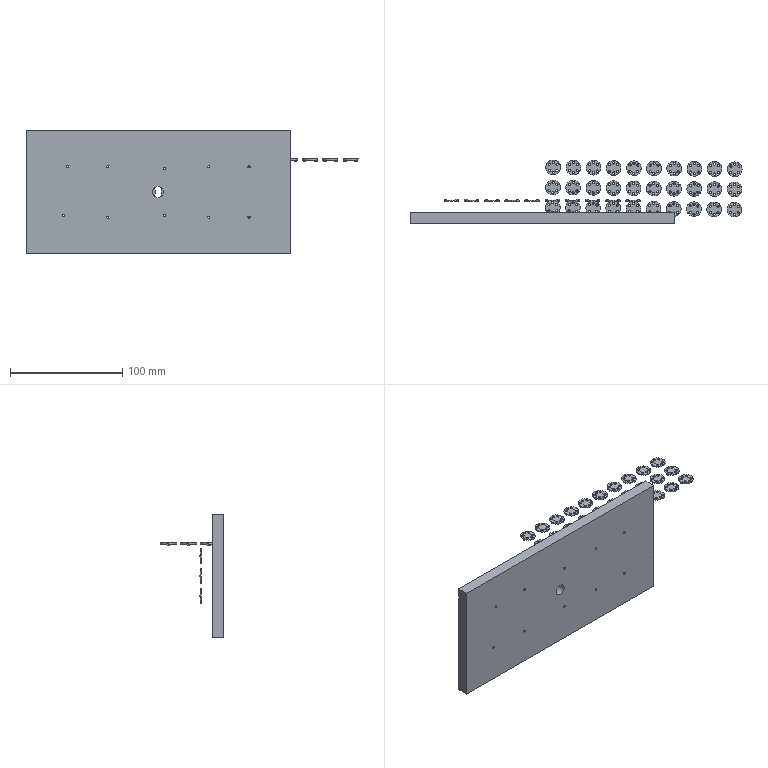NC program | NX | posted with a generic post | part box 296.27 x 56.878 x 110 mm
Lines 2497 to 3687 of 20851:
(DRILLING , TOOL : DK-Ø3)
N4992 T04 M6
N4994 G53
N4996 G17 G0 G90 X6.362 Y20.807 B0. C0. S1500 M3
N4998 G43 Z5. H4
N5000 G94 G81 G99 Z-1. F100. R1.
N5002 G0 Z5.
N5004 G81 X6.321 Y15.012 Z-1. R1.
N5006 G0 Z5.
N5008 G81 X9.826 Y22.378 Z-1. R1.
N5010 G0 Z5.
N5012 G81 X9.731 Y13.378 Z-1. R1.
N5014 G0 Z5.
N5016 G81 X13.195 Y14.949 Z-1. R1.
N5018 G0 Z5.
N5020 G81 X13.276 Y20.724 Z-1. R1.
N5022 G0 Z5.
N5024 G81 X24.361 Y20.617 Z-1. R1.
N5026 G0 Z5.
N5028 G81 X24.32 Y14.822 Z-1. R1.
N5030 G0 Z5.
N5032 G81 X27.825 Y22.188 Z-1. R1.
N5034 G0 Z5.
N5036 G81 X27.73 Y13.189 Z-1. R1.
N5038 G0 Z5.
N5040 G81 X31.194 Y14.76 Z-1. R1.
N5042 G0 Z5.
N5044 G81 X31.275 Y20.534 Z-1. R1.
N5046 G0 Z5.
N5048 G81 X42.36 Y20.427 Z-1. R1.
N5050 G0 Z5.
N5052 G81 X42.319 Y14.633 Z-1. R1.
N5054 G0 Z5.
N5056 G81 X45.824 Y21.998 Z-1. R1.
N5058 G0 Z5.
N5060 G81 X45.729 Y12.999 Z-1. R1.
N5062 G0 Z5.
N5064 G81 X49.193 Y14.57 Z-1. R1.
N5066 G0 Z5.
N5068 G81 X49.274 Y20.345 Z-1. R1.
N5070 G0 Z5.
N5072 G81 X60.359 Y20.238 Z-1. R1.
N5074 G0 Z5.
N5076 G81 X60.318 Y14.443 Z-1. R1.
N5078 G0 Z5.
N5080 G81 X63.823 Y21.809 Z-1. R1.
N5082 G0 Z5.
N5084 G81 X63.728 Y12.809 Z-1. R1.
N5086 G0 Z5.
N5088 G81 X67.192 Y14.38 Z-1. R1.
N5090 G0 Z5.
N5092 G81 X67.273 Y20.155 Z-1. R1.
N5094 G0 Z5.
N5096 G81 X78.358 Y20.048 Z-1. R1.
N5098 G0 Z5.
N5100 G81 X78.317 Y14.253 Z-1. R1.
N5102 G0 Z5.
N5104 G81 X81.822 Y21.619 Z-1. R1.
N5106 G0 Z5.
N5108 G81 X81.727 Y12.62 Z-1. R1.
N5110 G0 Z5.
N5112 G81 X85.191 Y14.191 Z-1. R1.
N5114 G0 Z5.
N5116 G81 X85.272 Y19.966 Z-1. R1.
N5118 G0 Z5.
N5120 G81 X96.357 Y19.859 Z-1. R1.
N5122 G0 Z5.
N5124 G81 X96.316 Y14.064 Z-1. R1.
N5126 G0 Z5.
N5128 G81 X99.821 Y21.43 Z-1. R1.
N5130 G0 Z5.
N5132 G81 X99.726 Y12.43 Z-1. R1.
N5134 G0 Z5.
N5136 G81 X103.19 Y14.001 Z-1. R1.
N5138 G0 Z5.
N5140 G81 X103.271 Y19.776 Z-1. R1.
N5142 G0 Z5.
N5144 G81 X114.356 Y19.669 Z-1. R1.
N5146 G0 Z5.
N5148 G81 X114.315 Y13.874 Z-1. R1.
N5150 G0 Z5.
N5152 G81 X117.82 Y21.24 Z-1. R1.
N5154 G0 Z5.
N5156 G81 X117.725 Y12.24 Z-1. R1.
N5158 G0 Z5.
N5160 G81 X121.189 Y13.811 Z-1. R1.
N5162 G0 Z5.
N5164 G81 X121.27 Y19.586 Z-1. R1.
N5166 G0 Z5.
N5168 G81 X132.355 Y19.479 Z-1. R1.
N5170 G0 Z5.
N5172 G81 X132.314 Y13.685 Z-1. R1.
N5174 G0 Z5.
N5176 G81 X135.819 Y21.05 Z-1. R1.
N5178 G0 Z5.
N5180 G81 X135.724 Y12.051 Z-1. R1.
N5182 G0 Z5.
N5184 G81 X139.188 Y13.622 Z-1. R1.
N5186 G0 Z5.
N5188 G81 X139.269 Y19.397 Z-1. R1.
N5190 G0 Z5.
N5192 G81 X150.354 Y19.29 Z-1. R1.
N5194 G0 Z5.
N5196 G81 X150.313 Y13.495 Z-1. R1.
N5198 G0 Z5.
N5200 G81 X153.818 Y20.861 Z-1. R1.
N5202 G0 Z5.
N5204 G81 X153.723 Y11.861 Z-1. R1.
N5206 G0 Z5.
N5208 G81 X157.187 Y13.432 Z-1. R1.
N5210 G0 Z5.
N5212 G81 X157.268 Y19.207 Z-1. R1.
N5214 G0 Z5.
N5216 G81 X168.353 Y19.1 Z-1. R1.
N5218 G0 Z5.
N5220 G81 X168.312 Y13.305 Z-1. R1.
N5222 G0 Z5.
N5224 G81 X171.817 Y20.671 Z-1. R1.
N5226 G0 Z5.
N5228 G81 X171.722 Y11.672 Z-1. R1.
N5230 G0 Z5.
N5232 G81 X175.186 Y13.243 Z-1. R1.
N5234 G0 Z5.
N5236 G81 X175.267 Y19.017 Z-1. R1.
N5238 G0 Z5.
N5240 G81 X168.163 Y1.101 Z-1. R1.
N5242 G0 Z5.
N5244 G81 X168.122 Y-4.694 Z-1. R1.
N5246 G0 Z5.
N5248 G81 X171.627 Y2.672 Z-1. R1.
N5250 G0 Z5.
N5252 G81 X171.533 Y-6.327 Z-1. R1.
N5254 G0 Z5.
N5256 G81 X174.996 Y-4.756 Z-1. R1.
N5258 G0 Z5.
N5260 G81 X175.077 Y1.018 Z-1. R1.
N5262 G0 Z5.
N5264 G81 X150.164 Y1.291 Z-1. R1.
N5266 G0 Z5.
N5268 G81 X150.123 Y-4.504 Z-1. R1.
N5270 G0 Z5.
N5272 G81 X153.628 Y2.862 Z-1. R1.
N5274 G0 Z5.
N5276 G81 X153.534 Y-6.138 Z-1. R1.
N5278 G0 Z5.
N5280 G81 X156.997 Y-4.567 Z-1. R1.
N5282 G0 Z5.
N5284 G81 X157.078 Y1.208 Z-1. R1.
N5286 G0 Z5.
N5288 G81 X132.165 Y1.48 Z-1. R1.
N5290 G0 Z5.
N5292 G81 X132.124 Y-4.314 Z-1. R1.
N5294 G0 Z5.
N5296 G81 X135.629 Y3.051 Z-1. R1.
N5298 G0 Z5.
N5300 G81 X135.535 Y-5.948 Z-1. R1.
N5302 G0 Z5.
N5304 G81 X138.998 Y-4.377 Z-1. R1.
N5306 G0 Z5.
N5308 G81 X139.079 Y1.398 Z-1. R1.
N5310 G0 Z5.
N5312 G81 X114.166 Y1.67 Z-1. R1.
N5314 G0 Z5.
N5316 G81 X114.125 Y-4.125 Z-1. R1.
N5318 G0 Z5.
N5320 G81 X117.63 Y3.241 Z-1. R1.
N5322 G0 Z5.
N5324 G81 X117.536 Y-5.759 Z-1. R1.
N5326 G0 Z5.
N5328 G81 X120.999 Y-4.188 Z-1. R1.
N5330 G0 Z5.
N5332 G81 X121.08 Y1.587 Z-1. R1.
N5334 G0 Z5.
N5336 G81 X96.167 Y1.86 Z-1. R1.
N5338 G0 Z5.
N5340 G81 X96.126 Y-3.935 Z-1. R1.
N5342 G0 Z5.
N5344 G81 X99.631 Y3.431 Z-1. R1.
N5346 G0 Z5.
N5348 G81 X99.537 Y-5.569 Z-1. R1.
N5350 G0 Z5.
N5352 G81 X103. Y-3.998 Z-1. R1.
N5354 G0 Z5.
N5356 G81 X103.081 Y1.777 Z-1. R1.
N5358 G0 Z5.
N5360 G81 X78.168 Y2.049 Z-1. R1.
N5362 G0 Z5.
N5364 G81 X78.127 Y-3.746 Z-1. R1.
N5366 G0 Z5.
N5368 G81 X81.632 Y3.62 Z-1. R1.
N5370 G0 Z5.
N5372 G81 X81.538 Y-5.379 Z-1. R1.
N5374 G0 Z5.
N5376 G81 X85.001 Y-3.808 Z-1. R1.
N5378 G0 Z5.
N5380 G81 X85.082 Y1.967 Z-1. R1.
N5382 G0 Z5.
N5384 G81 X60.169 Y2.239 Z-1. R1.
N5386 G0 Z5.
N5388 G81 X60.128 Y-3.556 Z-1. R1.
N5390 G0 Z5.
N5392 G81 X63.633 Y3.81 Z-1. R1.
N5394 G0 Z5.
N5396 G81 X63.539 Y-5.19 Z-1. R1.
N5398 G0 Z5.
N5400 G81 X67.002 Y-3.619 Z-1. R1.
N5402 G0 Z5.
N5404 G81 X67.083 Y2.156 Z-1. R1.
N5406 G0 Z5.
N5408 G81 X42.17 Y2.428 Z-1. R1.
N5410 G0 Z5.
N5412 G81 X42.129 Y-3.366 Z-1. R1.
N5414 G0 Z5.
N5416 G81 X45.634 Y3.999 Z-1. R1.
N5418 G0 Z5.
N5420 G81 X45.54 Y-5. Z-1. R1.
N5422 G0 Z5.
N5424 G81 X49.003 Y-3.429 Z-1. R1.
N5426 G0 Z5.
N5428 G81 X49.084 Y2.346 Z-1. R1.
N5430 G0 Z5.
N5432 G81 X24.171 Y2.618 Z-1. R1.
N5434 G0 Z5.
N5436 G81 X24.13 Y-3.177 Z-1. R1.
N5438 G0 Z5.
N5440 G81 X27.635 Y4.189 Z-1. R1.
N5442 G0 Z5.
N5444 G81 X27.541 Y-4.81 Z-1. R1.
N5446 G0 Z5.
N5448 G81 X31.004 Y-3.239 Z-1. R1.
N5450 G0 Z5.
N5452 G81 X31.085 Y2.535 Z-1. R1.
N5454 G0 Z5.
N5456 G81 X6.172 Y2.808 Z-1. R1.
N5458 G0 Z5.
N5460 G81 X6.131 Y-2.987 Z-1. R1.
N5462 G0 Z5.
N5464 G81 X9.636 Y4.379 Z-1. R1.
N5466 G0 Z5.
N5468 G81 X9.542 Y-4.621 Z-1. R1.
N5470 G0 Z5.
N5472 G81 X13.005 Y-3.05 Z-1. R1.
N5474 G0 Z5.
N5476 G81 X13.086 Y2.725 Z-1. R1.
N5478 G0 Z5.
N5480 G81 X5.983 Y-15.191 Z-1. R1.
N5482 G0 Z5.
N5484 G81 X5.942 Y-20.986 Z-1. R1.
N5486 G0 Z5.
N5488 G81 X9.447 Y-13.62 Z-1. R1.
N5490 G0 Z5.
N5492 G81 X9.352 Y-22.62 Z-1. R1.
N5494 G0 Z5.
N5496 G81 X12.816 Y-21.049 Z-1. R1.
N5498 G0 Z5.
N5500 G81 X12.897 Y-15.274 Z-1. R1.
N5502 G0 Z5.
N5504 G81 X23.982 Y-15.381 Z-1. R1.
N5506 G0 Z5.
N5508 G81 X23.941 Y-21.176 Z-1. R1.
N5510 G0 Z5.
N5512 G81 X27.446 Y-13.81 Z-1. R1.
N5514 G0 Z5.
N5516 G81 X27.351 Y-22.809 Z-1. R1.
N5518 G0 Z5.
N5520 G81 X30.815 Y-21.238 Z-1. R1.
N5522 G0 Z5.
N5524 G81 X30.896 Y-15.464 Z-1. R1.
N5526 G0 Z5.
N5528 G81 X41.981 Y-15.571 Z-1. R1.
N5530 G0 Z5.
N5532 G81 X41.94 Y-21.365 Z-1. R1.
N5534 G0 Z5.
N5536 G81 X45.445 Y-14. Z-1. R1.
N5538 G0 Z5.
N5540 G81 X45.35 Y-22.999 Z-1. R1.
N5542 G0 Z5.
N5544 G81 X48.814 Y-21.428 Z-1. R1.
N5546 G0 Z5.
N5548 G81 X48.895 Y-15.653 Z-1. R1.
N5550 G0 Z5.
N5552 G81 X59.98 Y-15.76 Z-1. R1.
N5554 G0 Z5.
N5556 G81 X59.939 Y-21.555 Z-1. R1.
N5558 G0 Z5.
N5560 G81 X63.444 Y-14.189 Z-1. R1.
N5562 G0 Z5.
N5564 G81 X63.349 Y-23.189 Z-1. R1.
N5566 G0 Z5.
N5568 G81 X66.813 Y-21.618 Z-1. R1.
N5570 G0 Z5.
N5572 G81 X66.894 Y-15.843 Z-1. R1.
N5574 G0 Z5.
N5576 G81 X77.979 Y-15.95 Z-1. R1.
N5578 G0 Z5.
N5580 G81 X77.938 Y-21.745 Z-1. R1.
N5582 G0 Z5.
N5584 G81 X81.443 Y-14.379 Z-1. R1.
N5586 G0 Z5.
N5588 G81 X81.348 Y-23.378 Z-1. R1.
N5590 G0 Z5.
N5592 G81 X84.812 Y-21.807 Z-1. R1.
N5594 G0 Z5.
N5596 G81 X84.893 Y-16.032 Z-1. R1.
N5598 G0 Z5.
N5600 G81 X95.978 Y-16.139 Z-1. R1.
N5602 G0 Z5.
N5604 G81 X95.937 Y-21.934 Z-1. R1.
N5606 G0 Z5.
N5608 G81 X99.442 Y-14.568 Z-1. R1.
N5610 G0 Z5.
N5612 G81 X99.347 Y-23.568 Z-1. R1.
N5614 G0 Z5.
N5616 G81 X102.811 Y-21.997 Z-1. R1.
N5618 G0 Z5.
N5620 G81 X102.892 Y-16.222 Z-1. R1.
N5622 G0 Z5.
N5624 G81 X113.977 Y-16.329 Z-1. R1.
N5626 G0 Z5.
N5628 G81 X113.936 Y-22.124 Z-1. R1.
N5630 G0 Z5.
N5632 G81 X117.441 Y-14.758 Z-1. R1.
N5634 G0 Z5.
N5636 G81 X117.346 Y-23.758 Z-1. R1.
N5638 G0 Z5.
N5640 G81 X120.81 Y-22.187 Z-1. R1.
N5642 G0 Z5.
N5644 G81 X120.891 Y-16.412 Z-1. R1.
N5646 G0 Z5.
N5648 G81 X131.976 Y-16.519 Z-1. R1.
N5650 G0 Z5.
N5652 G81 X131.935 Y-22.313 Z-1. R1.
N5654 G0 Z5.
N5656 G81 X135.44 Y-14.948 Z-1. R1.
N5658 G0 Z5.
N5660 G81 X135.345 Y-23.947 Z-1. R1.
N5662 G0 Z5.
N5664 G81 X138.809 Y-22.376 Z-1. R1.
N5666 G0 Z5.
N5668 G81 X138.89 Y-16.601 Z-1. R1.
N5670 G0 Z5.
N5672 G81 X149.975 Y-16.708 Z-1. R1.
N5674 G0 Z5.
N5676 G81 X149.934 Y-22.503 Z-1. R1.
N5678 G0 Z5.
N5680 G81 X153.439 Y-15.137 Z-1. R1.
N5682 G0 Z5.
N5684 G81 X153.344 Y-24.137 Z-1. R1.
N5686 G0 Z5.
N5688 G81 X156.808 Y-22.566 Z-1. R1.
N5690 G0 Z5.
N5692 G81 X156.889 Y-16.791 Z-1. R1.
N5694 G0 Z5.
N5696 G81 X167.974 Y-16.898 Z-1. R1.
N5698 G0 Z5.
N5700 G81 X167.933 Y-22.693 Z-1. R1.
N5702 G0 Z5.
N5704 G81 X171.438 Y-15.327 Z-1. R1.
N5706 G0 Z5.
N5708 G81 X171.343 Y-24.326 Z-1. R1.
N5710 G0 Z5.
N5712 G81 X174.807 Y-22.755 Z-1. R1.
N5714 G0 Z5.
N5716 G81 X174.888 Y-16.981 Z-1. R1.
N5718 G0 Z5.
N5720 G80
N5722 G0 X174.888 Y-16.981 Z5.
(PLANAR_MILL_COPY_1_COPY_10 , TOOL : DK-Ø3)
N5724 Z10. S5000
N5726 X179.768 Y17.154
N5728 G1 Z-0.4 F5000.
N5730 G41 X179.67 Y17.171 F800. D4
N5732 G3 X178.67 Y16.171 R1.
N5734 G2 X171.77 Y9.271 R6.9
N5736 X178.67 Y16.171 R-6.9
N5738 G1 X178.669 Y16.071
N5740 G3 X179.654 Y15.057 R1.
N5742 G40
N5744 G1 X179.753 Y15.073
N5746 G0 Z3.
N5748 X179.578 Y-0.845
N5750 G1 Z-0.4 F5000.
N5752 G41 X179.48 Y-0.828 F800.
N5754 G3 X178.48 Y-1.828 R1.
N5756 G2 X171.58 Y-8.728 R6.9
N5758 X178.48 Y-1.828 R-6.9
N5760 G1 X178.479 Y-1.928
N5762 G3 X179.465 Y-2.942 R1.
N5764 G40
N5766 G1 X179.563 Y-2.926
N5768 G0 Z3.
N5770 X179.389 Y-18.844
N5772 G1 Z-0.4 F5000.
N5774 G41 X179.29 Y-18.827 F800.
N5776 G3 X178.29 Y-19.827 R1.
N5778 G2 X171.39 Y-26.727 R6.9
N5780 X178.29 Y-19.827 R-6.9
N5782 G1 Y-19.927
N5784 G3 X179.275 Y-20.941 R1.
N5786 G40
N5788 G1 X179.374 Y-20.925
N5790 G0 Z3.
N5792 X161.39 Y-18.654
N5794 G1 Z-0.4 F5000.
N5796 G41 X161.291 Y-18.637 F800.
N5798 G3 X160.291 Y-19.637 R1.
N5800 G2 X153.391 Y-26.537 R6.9
N5802 X160.291 Y-19.637 R-6.9
N5804 G1 Y-19.737
N5806 G3 X161.276 Y-20.751 R1.
N5808 G40
N5810 G1 X161.375 Y-20.736
N5812 G0 Z3.
N5814 X161.579 Y-0.655
N5816 G1 Z-0.4 F5000.
N5818 G41 X161.481 Y-0.638 F800.
N5820 G3 X160.481 Y-1.638 R1.
N5822 G2 X153.581 Y-8.538 R6.9
N5824 X160.481 Y-1.638 R-6.9
N5826 G1 X160.48 Y-1.738
N5828 G3 X161.466 Y-2.752 R1.
N5830 G40
N5832 G1 X161.564 Y-2.737
N5834 G0 Z3.
N5836 X161.769 Y17.344
N5838 G1 Z-0.4 F5000.
N5840 G41 X161.671 Y17.361 F800.
N5842 G3 X160.671 Y16.361 R1.
N5844 G2 X153.771 Y9.461 R6.9
N5846 X160.671 Y16.361 R-6.9
N5848 G1 X160.67 Y16.261
N5850 G3 X161.655 Y15.247 R1.
N5852 G40
N5854 G1 X161.754 Y15.262
N5856 G0 Z3.
N5858 X143.77 Y17.533
N5860 G1 Z-0.4 F5000.
N5862 G41 X143.672 Y17.551 F800.
N5864 G3 X142.672 Y16.551 R1.
N5866 G2 X135.772 Y9.651 R6.9
N5868 X142.672 Y16.551 R-6.9
N5870 G1 X142.671 Y16.451
N5872 G3 X143.656 Y15.436 R1.
N5874 G40
N5876 G1 X143.755 Y15.452
N5878 G0 Z3.
N5880 X143.58 Y-0.466
N5882 G1 Z-0.4 F5000.
N5884 G41 X143.482 Y-0.448 F800.
N5886 G3 X142.482 Y-1.448 R1.
N5888 G2 X135.582 Y-8.348 R6.9
N5890 X142.482 Y-1.448 R-6.9
N5892 G1 X142.481 Y-1.548
N5894 G3 X143.467 Y-2.563 R1.
N5896 G40
N5898 G1 X143.565 Y-2.547
N5900 G0 Z3.
N5902 X143.391 Y-18.465
N5904 G1 Z-0.4 F5000.
N5906 G41 X143.292 Y-18.447 F800.
N5908 G3 X142.292 Y-19.447 R1.
N5910 G2 X135.392 Y-26.347 R6.9
N5912 X142.292 Y-19.447 R-6.9
N5914 G1 Y-19.547
N5916 G3 X143.277 Y-20.562 R1.
N5918 G40
N5920 G1 X143.376 Y-20.546
N5922 G0 Z3.
N5924 X125.392 Y-18.275
N5926 G1 Z-0.4 F5000.
N5928 G41 X125.293 Y-18.258 F800.
N5930 G3 X124.293 Y-19.258 R1.
N5932 G2 X117.393 Y-26.158 R6.9
N5934 X124.293 Y-19.258 R-6.9
N5936 G1 Y-19.358
N5938 G3 X125.278 Y-20.372 R1.
N5940 G40
N5942 G1 X125.377 Y-20.356
N5944 G0 Z3.
N5946 X125.581 Y-0.276
N5948 G1 Z-0.4 F5000.
N5950 G41 X125.483 Y-0.259 F800.
N5952 G3 X124.483 Y-1.259 R1.
N5954 G2 X117.583 Y-8.159 R6.9
N5956 X124.483 Y-1.259 R-6.9
N5958 G1 X124.482 Y-1.359
N5960 G3 X125.468 Y-2.373 R1.
N5962 G40
N5964 G1 X125.566 Y-2.357
N5966 G0 Z3.
N5968 X125.771 Y17.723
N5970 G1 Z-0.4 F5000.
N5972 G41 X125.673 Y17.74 F800.
N5974 G3 X124.673 Y16.74 R1.
N5976 G2 X117.773 Y9.84 R6.9
N5978 X124.673 Y16.74 R-6.9
N5980 G1 X124.672 Y16.64
N5982 G3 X125.657 Y15.626 R1.
N5984 G40
N5986 G1 X125.756 Y15.642
N5988 G0 Z3.
N5990 X107.772 Y17.912
N5992 G1 Z-0.4 F5000.
N5994 G41 X107.674 Y17.93 F800.
N5996 G3 X106.674 Y16.93 R1.
N5998 G2 X99.774 Y10.03 R6.9
N6000 X106.674 Y16.93 R-6.9
N6002 G1 X106.673 Y16.83
N6004 G3 X107.658 Y15.815 R1.
N6006 G40
N6008 G1 X107.757 Y15.831
N6010 G0 Z3.
N6012 X107.582 Y-0.087
N6014 G1 Z-0.4 F5000.
N6016 G41 X107.484 Y-0.069 F800.
N6018 G3 X106.484 Y-1.069 R1.
N6020 G2 X99.584 Y-7.969 R6.9
N6022 X106.484 Y-1.069 R-6.9
N6024 G1 X106.483 Y-1.169
N6026 G3 X107.469 Y-2.184 R1.
N6028 G40
N6030 G1 X107.567 Y-2.168
N6032 G0 Z3.
N6034 X107.393 Y-18.086
N6036 G1 Z-0.4 F5000.
N6038 G41 X107.294 Y-18.068 F800.
N6040 G3 X106.294 Y-19.068 R1.
N6042 G2 X99.394 Y-25.968 R6.9
N6044 X106.294 Y-19.068 R-6.9
N6046 G1 Y-19.168
N6048 G3 X107.279 Y-20.183 R1.
N6050 G40
N6052 G1 X107.378 Y-20.167
N6054 G0 Z3.
N6056 X89.394 Y-17.896
N6058 G1 Z-0.4 F5000.
N6060 G41 X89.295 Y-17.879 F800.
N6062 G3 X88.295 Y-18.879 R1.
N6064 G2 X81.395 Y-25.779 R6.9
N6066 X88.295 Y-18.879 R-6.9
N6068 G1 Y-18.979
N6070 G3 X89.28 Y-19.993 R1.
N6072 G40
N6074 G1 X89.379 Y-19.977
N6076 G0 Z3.
N6078 X89.583 Y0.103
N6080 G1 Z-0.4 F5000.
N6082 G41 X89.485 Y0.12 F800.
N6084 G3 X88.485 Y-0.88 R1.
N6086 G2 X81.585 Y-7.78 R6.9
N6088 X88.485 Y-0.88 R-6.9
N6090 G1 X88.484 Y-0.98
N6092 G3 X89.47 Y-1.994 R1.
N6094 G40
N6096 G1 X89.568 Y-1.978
N6098 G0 Z3.
N6100 X89.773 Y18.102
N6102 G1 Z-0.4 F5000.
N6104 G41 X89.675 Y18.119 F800.
N6106 G3 X88.675 Y17.119 R1.
N6108 G2 X81.775 Y10.219 R6.9
N6110 X88.675 Y17.119 R-6.9
N6112 G1 X88.674 Y17.019
N6114 G3 X89.659 Y16.005 R1.
N6116 G40
N6118 G1 X89.758 Y16.021
N6120 G0 Z3.
N6122 X71.774 Y18.292
N6124 G1 Z-0.4 F5000.
N6126 G41 X71.676 Y18.309 F800.
N6128 G3 X70.676 Y17.309 R1.
N6130 G2 X63.776 Y10.409 R6.9
N6132 X70.676 Y17.309 R-6.9
N6134 G1 X70.675 Y17.209
N6136 G3 X71.66 Y16.195 R1.
N6138 G40
N6140 G1 X71.759 Y16.211
N6142 G0 Z3.
N6144 X71.584 Y0.293
N6146 G1 Z-0.4 F5000.
N6148 G41 X71.486 Y0.31 F800.
N6150 G3 X70.486 Y-0.69 R1.
N6152 G2 X63.586 Y-7.59 R6.9
N6154 X70.486 Y-0.69 R-6.9
N6156 G1 X70.485 Y-0.79
N6158 G3 X71.471 Y-1.804 R1.
N6160 G40
N6162 G1 X71.569 Y-1.788
N6164 G0 Z3.
N6166 X71.395 Y-17.706
N6168 G1 Z-0.4 F5000.
N6170 G41 X71.296 Y-17.689 F800.
N6172 G3 X70.296 Y-18.689 R1.
N6174 G2 X63.396 Y-25.589 R6.9
N6176 X70.296 Y-18.689 R-6.9
N6178 G1 Y-18.789
N6180 G3 X71.281 Y-19.803 R1.
N6182 G40
N6184 G1 X71.38 Y-19.787
N6186 G0 Z3.
N6188 X53.396 Y-17.517
N6190 G1 Z-0.4 F5000.
N6192 G41 X53.297 Y-17.499 F800.
N6194 G3 X52.297 Y-18.499 R1.
N6196 G2 X45.397 Y-25.399 R6.9
N6198 X52.297 Y-18.499 R-6.9
N6200 G1 Y-18.599
N6202 G3 X53.282 Y-19.614 R1.
N6204 G40
N6206 G1 X53.381 Y-19.598
N6208 G0 Z3.
N6210 X53.585 Y0.482
N6212 G1 Z-0.4 F5000.
N6214 G41 X53.487 Y0.5 F800.
N6216 G3 X52.487 Y-0.5 R1.
N6218 G2 X45.587 Y-7.4 R6.9
N6220 X52.487 Y-0.5 R-6.9
N6222 G1 X52.486 Y-0.6
N6224 G3 X53.472 Y-1.615 R1.
N6226 G40
N6228 G1 X53.57 Y-1.599
N6230 G0 Z3.
N6232 X53.775 Y18.481
N6234 G1 Z-0.4 F5000.
N6236 G41 X53.677 Y18.499 F800.
N6238 G3 X52.677 Y17.499 R1.
N6240 G2 X45.777 Y10.599 R6.9
N6242 X52.677 Y17.499 R-6.9
N6244 G1 X52.676 Y17.399
N6246 G3 X53.661 Y16.384 R1.
N6248 G40
N6250 G1 X53.76 Y16.4
N6252 G0 Z3.
N6254 X35.776 Y18.671
N6256 G1 Z-0.4 F5000.
N6258 G41 X35.678 Y18.688 F800.
N6260 G3 X34.678 Y17.688 R1.
N6262 G2 X27.778 Y10.788 R6.9
N6264 X34.678 Y17.688 R-6.9
N6266 G1 X34.677 Y17.588
N6268 G3 X35.662 Y16.574 R1.
N6270 G40
N6272 G1 X35.761 Y16.59
N6274 G0 Z3.
N6276 X35.586 Y0.672
N6278 G1 Z-0.4 F5000.
N6280 G41 X35.488 Y0.689 F800.
N6282 G3 X34.488 Y-0.311 R1.
N6284 G2 X27.588 Y-7.211 R6.9
N6286 X34.488 Y-0.311 R-6.9
N6288 G1 X34.487 Y-0.411
N6290 G3 X35.473 Y-1.425 R1.
N6292 G40
N6294 G1 X35.571 Y-1.409
N6296 G0 Z3.
N6298 X35.397 Y-17.327
N6300 G1 Z-0.4 F5000.
N6302 G41 X35.298 Y-17.31 F800.
N6304 G3 X34.298 Y-18.31 R1.
N6306 G2 X27.398 Y-25.21 R6.9
N6308 X34.298 Y-18.31 R-6.9
N6310 G1 Y-18.41
N6312 G3 X35.283 Y-19.424 R1.
N6314 G40
N6316 G1 X35.382 Y-19.408
N6318 G0 Z3.
N6320 X17.398 Y-17.137
N6322 G1 Z-0.4 F5000.
N6324 G41 X17.299 Y-17.12 F800.
N6326 G3 X16.299 Y-18.12 R1.
N6328 G2 X9.399 Y-25.02 R6.9
N6330 X16.299 Y-18.12 R-6.9
N6332 G1 Y-18.22
N6334 G3 X17.284 Y-19.234 R1.
N6336 G40
N6338 G1 X17.383 Y-19.219
N6340 G0 Z3.
N6342 X17.587 Y0.862
N6344 G1 Z-0.4 F5000.
N6346 G41 X17.489 Y0.879 F800.
N6348 G3 X16.489 Y-0.121 R1.
N6350 G2 X9.589 Y-7.021 R6.9
N6352 X16.489 Y-0.121 R-6.9
N6354 G1 X16.488 Y-0.221
N6356 G3 X17.474 Y-1.235 R1.
N6358 G40
N6360 G1 X17.572 Y-1.22
N6362 G0 Z3.
N6364 X17.777 Y18.861
N6366 G1 Z-0.4 F5000.
N6368 G41 X17.679 Y18.878 F800.
N6370 G3 X16.679 Y17.878 R1.
N6372 G2 X9.779 Y10.978 R6.9
N6374 X16.679 Y17.878 R-6.9
N6376 G1 X16.678 Y17.778
N6378 G3 X17.663 Y16.764 R1.
N6380 G40
N6382 G1 X17.762 Y16.779
N6384 G0 Z10.
N6386 M5
(DRILLING_COPY , TOOL : D02钻头)
N6388 T05 M6
N6390 G53
N6392 G17 G0 G90 X6.362 Y20.807 B0. C0. S1500 M3
N6394 G43 Z5. H5
N6396 G94 G81 G99 Z-4. F100. R1.
N6398 G0 Z5.
N6400 G81 X6.321 Y15.012 Z-4. R1.
N6402 G0 Z5.
N6404 G81 X9.826 Y22.378 Z-4. R1.
N6406 G0 Z5.
N6408 G81 X9.731 Y13.378 Z-4. R1.
N6410 G0 Z5.
N6412 G81 X13.195 Y14.949 Z-4. R1.
N6414 G0 Z5.
N6416 G81 X13.276 Y20.724 Z-4. R1.
N6418 G0 Z5.
N6420 G81 X24.361 Y20.617 Z-4. R1.
N6422 G0 Z5.
N6424 G81 X24.32 Y14.822 Z-4. R1.
N6426 G0 Z5.
N6428 G81 X27.825 Y22.188 Z-4. R1.
N6430 G0 Z5.
N6432 G81 X27.73 Y13.189 Z-4. R1.
N6434 G0 Z5.
N6436 G81 X31.194 Y14.76 Z-4. R1.
N6438 G0 Z5.
N6440 G81 X31.275 Y20.534 Z-4. R1.
N6442 G0 Z5.
N6444 G81 X42.36 Y20.427 Z-4. R1.
N6446 G0 Z5.
N6448 G81 X42.319 Y14.633 Z-4. R1.
N6450 G0 Z5.
N6452 G81 X45.824 Y21.998 Z-4. R1.
N6454 G0 Z5.
N6456 G81 X45.729 Y12.999 Z-4. R1.
N6458 G0 Z5.
N6460 G81 X49.193 Y14.57 Z-4. R1.
N6462 G0 Z5.
N6464 G81 X49.274 Y20.345 Z-4. R1.
N6466 G0 Z5.
N6468 G81 X60.359 Y20.238 Z-4. R1.
N6470 G0 Z5.
N6472 G81 X60.318 Y14.443 Z-4. R1.
N6474 G0 Z5.
N6476 G81 X63.823 Y21.809 Z-4. R1.
N6478 G0 Z5.
N6480 G81 X63.728 Y12.809 Z-4. R1.
N6482 G0 Z5.
N6484 G81 X67.192 Y14.38 Z-4. R1.
N6486 G0 Z5.
N6488 G81 X67.273 Y20.155 Z-4. R1.
N6490 G0 Z5.
N6492 G81 X78.358 Y20.048 Z-4. R1.
N6494 G0 Z5.
N6496 G81 X78.317 Y14.253 Z-4. R1.
N6498 G0 Z5.
N6500 G81 X81.822 Y21.619 Z-4. R1.
N6502 G0 Z5.
N6504 G81 X81.727 Y12.62 Z-4. R1.
N6506 G0 Z5.
N6508 G81 X85.191 Y14.191 Z-4. R1.
N6510 G0 Z5.
N6512 G81 X85.272 Y19.966 Z-4. R1.
N6514 G0 Z5.
N6516 G81 X96.357 Y19.859 Z-4. R1.
N6518 G0 Z5.
N6520 G81 X96.316 Y14.064 Z-4. R1.
N6522 G0 Z5.
N6524 G81 X99.821 Y21.43 Z-4. R1.
N6526 G0 Z5.
N6528 G81 X99.726 Y12.43 Z-4. R1.
N6530 G0 Z5.
N6532 G81 X103.19 Y14.001 Z-4. R1.
N6534 G0 Z5.
N6536 G81 X103.271 Y19.776 Z-4. R1.
N6538 G0 Z5.
N6540 G81 X114.356 Y19.669 Z-4. R1.
N6542 G0 Z5.
N6544 G81 X114.315 Y13.874 Z-4. R1.
N6546 G0 Z5.
N6548 G81 X117.82 Y21.24 Z-4. R1.
N6550 G0 Z5.
N6552 G81 X117.725 Y12.24 Z-4. R1.
N6554 G0 Z5.
N6556 G81 X121.189 Y13.811 Z-4. R1.
N6558 G0 Z5.
N6560 G81 X121.27 Y19.586 Z-4. R1.
N6562 G0 Z5.
N6564 G81 X132.355 Y19.479 Z-4. R1.
N6566 G0 Z5.
N6568 G81 X132.314 Y13.685 Z-4. R1.
N6570 G0 Z5.
N6572 G81 X135.819 Y21.05 Z-4. R1.
N6574 G0 Z5.
N6576 G81 X135.724 Y12.051 Z-4. R1.
N6578 G0 Z5.
N6580 G81 X139.188 Y13.622 Z-4. R1.
N6582 G0 Z5.
N6584 G81 X139.269 Y19.397 Z-4. R1.
N6586 G0 Z5.
N6588 G81 X150.354 Y19.29 Z-4. R1.
N6590 G0 Z5.
N6592 G81 X150.313 Y13.495 Z-4. R1.
N6594 G0 Z5.
N6596 G81 X153.818 Y20.861 Z-4. R1.
N6598 G0 Z5.
N6600 G81 X153.723 Y11.861 Z-4. R1.
N6602 G0 Z5.
N6604 G81 X157.187 Y13.432 Z-4. R1.
N6606 G0 Z5.
N6608 G81 X157.268 Y19.207 Z-4. R1.
N6610 G0 Z5.
N6612 G81 X168.353 Y19.1 Z-4. R1.
N6614 G0 Z5.
N6616 G81 X168.312 Y13.305 Z-4. R1.
N6618 G0 Z5.
N6620 G81 X171.817 Y20.671 Z-4. R1.
N6622 G0 Z5.
N6624 G81 X171.722 Y11.672 Z-4. R1.
N6626 G0 Z5.
N6628 G81 X175.186 Y13.243 Z-4. R1.
N6630 G0 Z5.
N6632 G81 X175.267 Y19.017 Z-4. R1.
N6634 G0 Z5.
N6636 G81 X168.163 Y1.101 Z-4. R1.
N6638 G0 Z5.
N6640 G81 X168.122 Y-4.694 Z-4. R1.
N6642 G0 Z5.
N6644 G81 X171.627 Y2.672 Z-4. R1.
N6646 G0 Z5.
N6648 G81 X171.533 Y-6.327 Z-4. R1.
N6650 G0 Z5.
N6652 G81 X174.996 Y-4.756 Z-4. R1.
N6654 G0 Z5.
N6656 G81 X175.077 Y1.018 Z-4. R1.
N6658 G0 Z5.
N6660 G81 X150.164 Y1.291 Z-4. R1.
N6662 G0 Z5.
N6664 G81 X150.123 Y-4.504 Z-4. R1.
N6666 G0 Z5.
N6668 G81 X153.628 Y2.862 Z-4. R1.
N6670 G0 Z5.
N6672 G81 X153.534 Y-6.138 Z-4. R1.
N6674 G0 Z5.
N6676 G81 X156.997 Y-4.567 Z-4. R1.
N6678 G0 Z5.
N6680 G81 X157.078 Y1.208 Z-4. R1.
N6682 G0 Z5.
N6684 G81 X132.165 Y1.48 Z-4. R1.
N6686 G0 Z5.
N6688 G81 X132.124 Y-4.314 Z-4. R1.
N6690 G0 Z5.
N6692 G81 X135.629 Y3.051 Z-4. R1.
N6694 G0 Z5.
N6696 G81 X135.535 Y-5.948 Z-4. R1.
N6698 G0 Z5.
N6700 G81 X138.998 Y-4.377 Z-4. R1.
N6702 G0 Z5.
N6704 G81 X139.079 Y1.398 Z-4. R1.
N6706 G0 Z5.
N6708 G81 X114.166 Y1.67 Z-4. R1.
N6710 G0 Z5.
N6712 G81 X114.125 Y-4.125 Z-4. R1.
N6714 G0 Z5.
N6716 G81 X117.63 Y3.241 Z-4. R1.
N6718 G0 Z5.
N6720 G81 X117.536 Y-5.759 Z-4. R1.
N6722 G0 Z5.
N6724 G81 X120.999 Y-4.188 Z-4. R1.
N6726 G0 Z5.
N6728 G81 X121.08 Y1.587 Z-4. R1.
N6730 G0 Z5.
N6732 G81 X96.167 Y1.86 Z-4. R1.
N6734 G0 Z5.
N6736 G81 X96.126 Y-3.935 Z-4. R1.
N6738 G0 Z5.
N6740 G81 X99.631 Y3.431 Z-4. R1.
N6742 G0 Z5.
N6744 G81 X99.537 Y-5.569 Z-4. R1.
N6746 G0 Z5.
N6748 G81 X103. Y-3.998 Z-4. R1.
N6750 G0 Z5.
N6752 G81 X103.081 Y1.777 Z-4. R1.
N6754 G0 Z5.
N6756 G81 X78.168 Y2.049 Z-4. R1.
N6758 G0 Z5.
N6760 G81 X78.127 Y-3.746 Z-4. R1.
N6762 G0 Z5.
N6764 G81 X81.632 Y3.62 Z-4. R1.
N6766 G0 Z5.
N6768 G81 X81.538 Y-5.379 Z-4. R1.
N6770 G0 Z5.
N6772 G81 X85.001 Y-3.808 Z-4. R1.
N6774 G0 Z5.
N6776 G81 X85.082 Y1.967 Z-4. R1.
N6778 G0 Z5.
N6780 G81 X60.169 Y2.239 Z-4. R1.
N6782 G0 Z5.
N6784 G81 X60.128 Y-3.556 Z-4. R1.
N6786 G0 Z5.
N6788 G81 X63.633 Y3.81 Z-4. R1.
N6790 G0 Z5.
N6792 G81 X63.539 Y-5.19 Z-4. R1.
N6794 G0 Z5.
N6796 G81 X67.002 Y-3.619 Z-4. R1.
N6798 G0 Z5.
N6800 G81 X67.083 Y2.156 Z-4. R1.
N6802 G0 Z5.
N6804 G81 X42.17 Y2.428 Z-4. R1.
N6806 G0 Z5.
N6808 G81 X42.129 Y-3.366 Z-4. R1.
N6810 G0 Z5.
N6812 G81 X45.634 Y3.999 Z-4. R1.
N6814 G0 Z5.
N6816 G81 X45.54 Y-5. Z-4. R1.
N6818 G0 Z5.
N6820 G81 X49.003 Y-3.429 Z-4. R1.
N6822 G0 Z5.
N6824 G81 X49.084 Y2.346 Z-4. R1.
N6826 G0 Z5.
N6828 G81 X24.171 Y2.618 Z-4. R1.
N6830 G0 Z5.
N6832 G81 X24.13 Y-3.177 Z-4. R1.
N6834 G0 Z5.
N6836 G81 X27.635 Y4.189 Z-4. R1.
N6838 G0 Z5.
N6840 G81 X27.541 Y-4.81 Z-4. R1.
N6842 G0 Z5.
N6844 G81 X31.004 Y-3.239 Z-4. R1.
N6846 G0 Z5.
N6848 G81 X31.085 Y2.535 Z-4. R1.
N6850 G0 Z5.
N6852 G81 X6.172 Y2.808 Z-4. R1.
N6854 G0 Z5.
N6856 G81 X6.131 Y-2.987 Z-4. R1.
N6858 G0 Z5.
N6860 G81 X9.636 Y4.379 Z-4. R1.
N6862 G0 Z5.
N6864 G81 X9.542 Y-4.621 Z-4. R1.
N6866 G0 Z5.
N6868 G81 X13.005 Y-3.05 Z-4. R1.
N6870 G0 Z5.
N6872 G81 X13.086 Y2.725 Z-4. R1.
N6874 G0 Z5.
N6876 G81 X5.983 Y-15.191 Z-4. R1.
N6878 G0 Z5.
N6880 G81 X5.942 Y-20.986 Z-4. R1.
N6882 G0 Z5.
N6884 G81 X9.447 Y-13.62 Z-4. R1.
N6886 G0 Z5.
N6888 G81 X9.352 Y-22.62 Z-4. R1.
N6890 G0 Z5.
N6892 G81 X12.816 Y-21.049 Z-4. R1.
N6894 G0 Z5.
N6896 G81 X12.897 Y-15.274 Z-4. R1.
N6898 G0 Z5.
N6900 G81 X23.982 Y-15.381 Z-4. R1.
N6902 G0 Z5.
N6904 G81 X23.941 Y-21.176 Z-4. R1.
N6906 G0 Z5.
N6908 G81 X27.446 Y-13.81 Z-4. R1.
N6910 G0 Z5.
N6912 G81 X27.351 Y-22.809 Z-4. R1.
N6914 G0 Z5.
N6916 G81 X30.815 Y-21.238 Z-4. R1.
N6918 G0 Z5.
N6920 G81 X30.896 Y-15.464 Z-4. R1.
N6922 G0 Z5.
N6924 G81 X41.981 Y-15.571 Z-4. R1.
N6926 G0 Z5.
N6928 G81 X41.94 Y-21.365 Z-4. R1.
N6930 G0 Z5.
N6932 G81 X45.445 Y-14. Z-4. R1.
N6934 G0 Z5.
N6936 G81 X45.35 Y-22.999 Z-4. R1.
N6938 G0 Z5.
N6940 G81 X48.814 Y-21.428 Z-4. R1.
N6942 G0 Z5.
N6944 G81 X48.895 Y-15.653 Z-4. R1.
N6946 G0 Z5.
N6948 G81 X59.98 Y-15.76 Z-4. R1.
N6950 G0 Z5.
N6952 G81 X59.939 Y-21.555 Z-4. R1.
N6954 G0 Z5.
N6956 G81 X63.444 Y-14.189 Z-4. R1.
N6958 G0 Z5.
N6960 G81 X63.349 Y-23.189 Z-4. R1.
N6962 G0 Z5.
N6964 G81 X66.813 Y-21.618 Z-4. R1.
N6966 G0 Z5.
N6968 G81 X66.894 Y-15.843 Z-4. R1.
N6970 G0 Z5.
N6972 G81 X77.979 Y-15.95 Z-4. R1.
N6974 G0 Z5.
N6976 G81 X77.938 Y-21.745 Z-4. R1.
N6978 G0 Z5.
N6980 G81 X81.443 Y-14.379 Z-4. R1.
N6982 G0 Z5.
N6984 G81 X81.348 Y-23.378 Z-4. R1.
N6986 G0 Z5.
N6988 G81 X84.812 Y-21.807 Z-4. R1.
N6990 G0 Z5.
N6992 G81 X84.893 Y-16.032 Z-4. R1.
N6994 G0 Z5.
N6996 G81 X95.978 Y-16.139 Z-4. R1.
N6998 G0 Z5.
N7000 G81 X95.937 Y-21.934 Z-4. R1.
N7002 G0 Z5.
N7004 G81 X99.442 Y-14.568 Z-4. R1.
N7006 G0 Z5.
N7008 G81 X99.347 Y-23.568 Z-4. R1.
N7010 G0 Z5.
N7012 G81 X102.811 Y-21.997 Z-4. R1.
N7014 G0 Z5.
N7016 G81 X102.892 Y-16.222 Z-4. R1.
N7018 G0 Z5.
N7020 G81 X113.977 Y-16.329 Z-4. R1.
N7022 G0 Z5.
N7024 G81 X113.936 Y-22.124 Z-4. R1.
N7026 G0 Z5.
N7028 G81 X117.441 Y-14.758 Z-4. R1.
N7030 G0 Z5.
N7032 G81 X117.346 Y-23.758 Z-4. R1.
N7034 G0 Z5.
N7036 G81 X120.81 Y-22.187 Z-4. R1.
N7038 G0 Z5.
N7040 G81 X120.891 Y-16.412 Z-4. R1.
N7042 G0 Z5.
N7044 G81 X131.976 Y-16.519 Z-4. R1.
N7046 G0 Z5.
N7048 G81 X131.935 Y-22.313 Z-4. R1.
N7050 G0 Z5.
N7052 G81 X135.44 Y-14.948 Z-4. R1.
N7054 G0 Z5.
N7056 G81 X135.345 Y-23.947 Z-4. R1.
N7058 G0 Z5.
N7060 G81 X138.809 Y-22.376 Z-4. R1.
N7062 G0 Z5.
N7064 G81 X138.89 Y-16.601 Z-4. R1.
N7066 G0 Z5.
N7068 G81 X149.975 Y-16.708 Z-4. R1.
N7070 G0 Z5.
N7072 G81 X149.934 Y-22.503 Z-4. R1.
N7074 G0 Z5.
N7076 G81 X153.439 Y-15.137 Z-4. R1.
N7078 G0 Z5.
N7080 G81 X153.344 Y-24.137 Z-4. R1.
N7082 G0 Z5.
N7084 G81 X156.808 Y-22.566 Z-4. R1.
N7086 G0 Z5.
N7088 G81 X156.889 Y-16.791 Z-4. R1.
N7090 G0 Z5.
N7092 G81 X167.974 Y-16.898 Z-4. R1.
N7094 G0 Z5.
N7096 G81 X167.933 Y-22.693 Z-4. R1.
N7098 G0 Z5.
N7100 G81 X171.438 Y-15.327 Z-4. R1.
N7102 G0 Z5.
N7104 G81 X171.343 Y-24.326 Z-4. R1.
N7106 G0 Z5.
N7108 G81 X174.807 Y-22.755 Z-4. R1.
N7110 G0 Z5.
N7112 G81 X174.888 Y-16.981 Z-4. R1.
N7114 G0 Z5.
N7116 G80
N7118 G0 X174.888 Y-16.981 Z5.
N7120 M5
(PLANAR_MILL_3 , TOOL : D16)
N7122 T15 M6
N7124 G53
N7126 G17 G0 G90 X193.889 Y-20.064 B0. C0. S3500 M3
N7128 G43 Z10. H15
N7130 Z3.
N7132 G94 G1 Z0. F400.
N7134 X177.89 Y-19.895
N7136 X2.9 Y-18.052
N7138 X-13.099 Y-17.883
N7140 Z3.
N7142 G0 Z10.
N7144 X194.079 Y-2.065
N7146 Z3.
N7148 G1 Z0.
N7150 X178.08 Y-1.896
N7152 X3.089 Y-0.053
N7154 X-12.91 Y0.116
N7156 Z3.
N7158 G0 Z10.
N7160 X194.268 Y15.934
N7162 Z3.
N7164 G1 Z0.
N7166 X178.269 Y16.103
N7168 X3.279 Y17.946
N7170 X-12.72 Y18.115
N7172 Z3.
N7174 G0 Z10.
N7176 M5
(FACE_MILLING_1_COPY_1 , TOOL : D10R0)
N7178 T01 M6
N7180 G54
N7182 G17 G0 G90 X102.5 Y-22.125 B0. C0. S2200 M3
N7184 G43 Z50. H1
N7186 G94 G1 Z0.35 F5000.
N7188 X92.5 F1200.
N7190 X-92.5
N7192 Y-14.75
N7194 X92.5
N7196 Y-7.375
N7198 X-92.5
N7200 Y0.
N7202 X92.5
N7204 Y7.375
N7206 X-92.5
N7208 Y14.75
N7210 X92.5
N7212 Y22.125
N7214 X-92.5
N7216 X-102.5
N7218 G0 Z10.5
N7220 X102.5 Y-22.125
N7222 G1 Z0.2 F5000.
N7224 X92.5 F1200.
N7226 X-92.5
N7228 Y-14.75
N7230 X92.5
N7232 Y-7.375
N7234 X-92.5
N7236 Y0.
N7238 X92.5
N7240 Y7.375
N7242 X-92.5
N7244 Y14.75
N7246 X92.5
N7248 Y22.125
N7250 X-92.5
N7252 X-102.5
N7254 G0 Z10.5
N7256 X102.5 Y-22.125
N7258 G1 Z0.05 F5000.
N7260 X92.5 F1200.
N7262 X-92.5
N7264 Y-14.75
N7266 X92.5
N7268 Y-7.375
N7270 X-92.5
N7272 Y0.
N7274 X92.5
N7276 Y7.375
N7278 X-92.5
N7280 Y14.75
N7282 X92.5
N7284 Y22.125
N7286 X-92.5
N7288 X-102.5
N7290 G0 Z50.
(PLANAR_MILL_COPY , TOOL : D5R0)
N7292 T07 M6
N7294 G17 G43 G0 G90 X-72.4 Y-21.35 Z0.5 B0. C0. S3500 H7 M3
N7296 G94 G1 Z-0.5 F5000.
N7298 Z-1. F200.
N7300 G41 Y-20.85 D7
N7302 X-79.6
N7304 Y-15.15
N7306 X-72.4
N7308 Y-20.85
N7310 G40
N7312 X-71.9
N7314 Z-0.5
N7316 G0 X-82.4 Y-21.35
N7318 G1 Z-1.
N7320 G41 Y-20.85
N7322 X-89.6
N7324 Y-15.15
N7326 X-82.4
N7328 Y-20.85
N7330 G40
N7332 X-81.9
N7334 Z-0.5
N7336 G0 Z0.5